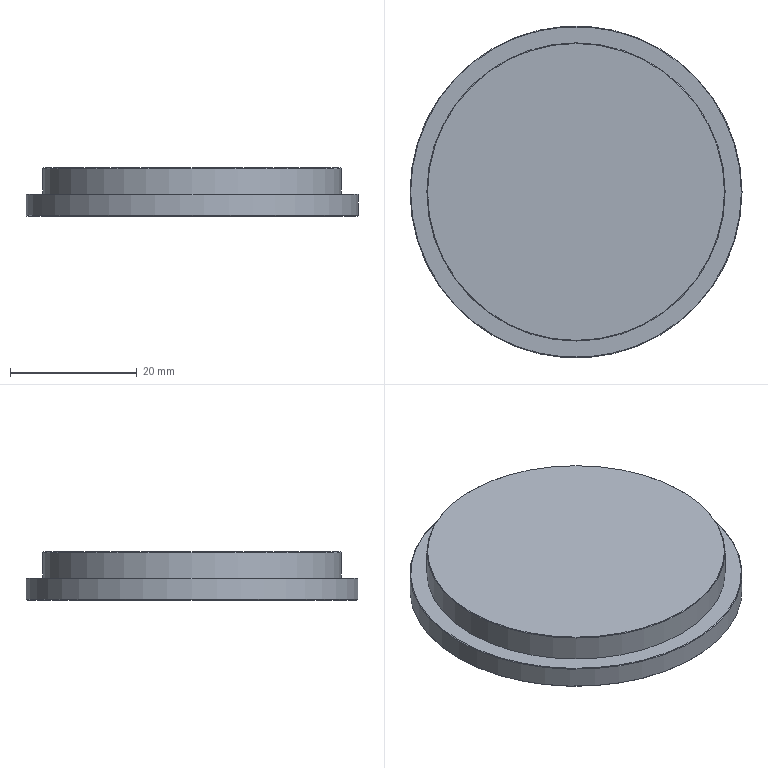Part | NX | features CHAMFER 4, DATUM_CSYS 4, EXTRUDE 3, SKETCH 3, DATUM_PLANE 2 | 1 solid | 11 faces | box 52.42 x 52.42 x 7.62 mm | volume 11135 mm3 | plane 4 | cone 4 | cylinder 3 | commonest cylinder face diameters 36.4 x1 47.08 x1 52.42 x1
STEP:
#1=CARTESIAN_POINT('',(-26.21,0.,0.1));
#2=VERTEX_POINT('',#1);
#3=CARTESIAN_POINT('',(0.,0.,0.1));
#4=DIRECTION('',(0.,0.,-1.));
#5=DIRECTION('',(-1.,0.,0.));
#6=AXIS2_PLACEMENT_3D('',#3,#4,#5);
#7=CIRCLE('',#6,26.21);
#8=EDGE_CURVE('',#2,#2,#7,.F.);
#9=ORIENTED_EDGE('',*,*,#8,.T.);
#10=EDGE_LOOP('',(#9));
#11=FACE_BOUND('',#10,.T.);
#12=CARTESIAN_POINT('',(-26.21,0.,3.38));
#13=VERTEX_POINT('',#12);
#14=CARTESIAN_POINT('',(0.,0.,3.38));
#15=DIRECTION('',(0.,0.,-1.));
#16=DIRECTION('',(-1.,0.,0.));
#17=AXIS2_PLACEMENT_3D('',#14,#15,#16);
#18=CIRCLE('',#17,26.21);
#19=EDGE_CURVE('',#13,#13,#18,.T.);
#20=ORIENTED_EDGE('',*,*,#19,.T.);
#21=EDGE_LOOP('',(#20));
#22=FACE_BOUND('',#21,.T.);
#23=CARTESIAN_POINT('',(0.,0.,7.62));
#24=DIRECTION('',(0.,0.,-1.));
#25=DIRECTION('',(-1.,0.,0.));
#26=AXIS2_PLACEMENT_3D('',#23,#24,#25);
#27=CYLINDRICAL_SURFACE('',#26,26.21);
#28=ADVANCED_FACE('',(#11,#22),#27,.T.);
#29=CARTESIAN_POINT('',(-18.3,0.,0.));
#30=VERTEX_POINT('',#29);
#31=CARTESIAN_POINT('',(0.,0.,0.));
#32=DIRECTION('',(0.,0.,-1.));
#33=DIRECTION('',(-1.,0.,0.));
#34=AXIS2_PLACEMENT_3D('',#31,#32,#33);
#35=CIRCLE('',#34,18.3);
#36=EDGE_CURVE('',#30,#30,#35,.F.);
#37=ORIENTED_EDGE('',*,*,#36,.T.);
#38=EDGE_LOOP('',(#37));
#39=FACE_BOUND('',#38,.T.);
#40=CARTESIAN_POINT('',(-26.11,0.,0.));
#41=VERTEX_POINT('',#40);
#42=CARTESIAN_POINT('',(0.,0.,0.));
#43=DIRECTION('',(0.,0.,-1.));
#44=DIRECTION('',(-1.,0.,0.));
#45=AXIS2_PLACEMENT_3D('',#42,#43,#44);
#46=CIRCLE('',#45,26.11);
#47=EDGE_CURVE('',#41,#41,#46,.T.);
#48=ORIENTED_EDGE('',*,*,#47,.T.);
#49=EDGE_LOOP('',(#48));
#50=FACE_BOUND('',#49,.T.);
#51=CARTESIAN_POINT('',(0.,0.,0.));
#52=DIRECTION('',(0.,0.,-1.));
#53=DIRECTION('',(-1.,0.,0.));
#54=AXIS2_PLACEMENT_3D('',#51,#52,#53);
#55=PLANE('',#54);
#56=ADVANCED_FACE('',(#39,#50),#55,.T.);
#57=CARTESIAN_POINT('',(-23.54,0.,7.52));
#58=VERTEX_POINT('',#57);
#59=CARTESIAN_POINT('',(0.,0.,7.52));
#60=DIRECTION('',(0.,0.,-1.));
#61=DIRECTION('',(-1.,0.,0.));
#62=AXIS2_PLACEMENT_3D('',#59,#60,#61);
#63=CIRCLE('',#62,23.54);
#64=EDGE_CURVE('',#58,#58,#63,.T.);
#65=ORIENTED_EDGE('',*,*,#64,.T.);
#66=EDGE_LOOP('',(#65));
#67=FACE_BOUND('',#66,.T.);
#68=CARTESIAN_POINT('',(23.54,0.,3.48));
#69=VERTEX_POINT('',#68);
#70=CARTESIAN_POINT('',(0.,0.,3.48));
#71=DIRECTION('',(0.,0.,-1.));
#72=DIRECTION('',(1.,0.,0.));
#73=AXIS2_PLACEMENT_3D('',#70,#71,#72);
#74=CIRCLE('',#73,23.54);
#75=EDGE_CURVE('',#69,#69,#74,.F.);
#76=ORIENTED_EDGE('',*,*,#75,.T.);
#77=EDGE_LOOP('',(#76));
#78=FACE_BOUND('',#77,.T.);
#79=CARTESIAN_POINT('',(0.,0.,3.48));
#80=DIRECTION('',(0.,0.,1.));
#81=DIRECTION('',(1.,0.,0.));
#82=AXIS2_PLACEMENT_3D('',#79,#80,#81);
#83=CYLINDRICAL_SURFACE('',#82,23.54);
#84=ADVANCED_FACE('',(#67,#78),#83,.T.);
#85=CARTESIAN_POINT('',(-26.11,0.,3.48));
#86=VERTEX_POINT('',#85);
#87=CARTESIAN_POINT('',(0.,0.,3.48));
#88=DIRECTION('',(0.,0.,-1.));
#89=DIRECTION('',(-1.,0.,0.));
#90=AXIS2_PLACEMENT_3D('',#87,#88,#89);
#91=CIRCLE('',#90,26.11);
#92=EDGE_CURVE('',#86,#86,#91,.F.);
#93=ORIENTED_EDGE('',*,*,#92,.T.);
#94=EDGE_LOOP('',(#93));
#95=FACE_BOUND('',#94,.T.);
#96=ORIENTED_EDGE('',*,*,#75,.F.);
#97=EDGE_LOOP('',(#96));
#98=FACE_BOUND('',#97,.T.);
#99=CARTESIAN_POINT('',(0.,0.,3.48));
#100=DIRECTION('',(0.,0.,-1.));
#101=DIRECTION('',(-1.,0.,0.));
#102=AXIS2_PLACEMENT_3D('',#99,#100,#101);
#103=PLANE('',#102);
#104=ADVANCED_FACE('',(#95,#98),#103,.F.);
#105=CARTESIAN_POINT('',(-23.44,0.,7.62));
#106=VERTEX_POINT('',#105);
#107=CARTESIAN_POINT('',(0.,0.,7.62));
#108=DIRECTION('',(0.,0.,-1.));
#109=DIRECTION('',(-1.,0.,0.));
#110=AXIS2_PLACEMENT_3D('',#107,#108,#109);
#111=CIRCLE('',#110,23.44);
#112=EDGE_CURVE('',#106,#106,#111,.F.);
#113=ORIENTED_EDGE('',*,*,#112,.T.);
#114=EDGE_LOOP('',(#113));
#115=FACE_BOUND('',#114,.T.);
#116=CARTESIAN_POINT('',(0.,0.,7.62));
#117=DIRECTION('',(0.,0.,-1.));
#118=DIRECTION('',(-1.,0.,0.));
#119=AXIS2_PLACEMENT_3D('',#116,#117,#118);
#120=PLANE('',#119);
#121=ADVANCED_FACE('',(#115),#120,.F.);
#122=CARTESIAN_POINT('',(-18.2,0.,0.1));
#123=VERTEX_POINT('',#122);
#124=CARTESIAN_POINT('',(0.,0.,0.1));
#125=DIRECTION('',(0.,0.,-1.));
#126=DIRECTION('',(-1.,0.,0.));
#127=AXIS2_PLACEMENT_3D('',#124,#125,#126);
#128=CIRCLE('',#127,18.2);
#129=EDGE_CURVE('',#123,#123,#128,.T.);
#130=ORIENTED_EDGE('',*,*,#129,.T.);
#131=EDGE_LOOP('',(#130));
#132=FACE_BOUND('',#131,.T.);
#133=CARTESIAN_POINT('',(18.2,0.,3.44));
#134=VERTEX_POINT('',#133);
#135=CARTESIAN_POINT('',(0.,0.,3.44));
#136=DIRECTION('',(0.,0.,1.));
#137=DIRECTION('',(1.,0.,0.));
#138=AXIS2_PLACEMENT_3D('',#135,#136,#137);
#139=CIRCLE('',#138,18.2);
#140=EDGE_CURVE('',#134,#134,#139,.F.);
#141=ORIENTED_EDGE('',*,*,#140,.F.);
#142=EDGE_LOOP('',(#141));
#143=FACE_BOUND('',#142,.T.);
#144=CARTESIAN_POINT('',(0.,0.,3.44));
#145=DIRECTION('',(0.,0.,-1.));
#146=DIRECTION('',(-1.,0.,0.));
#147=AXIS2_PLACEMENT_3D('',#144,#145,#146);
#148=CYLINDRICAL_SURFACE('',#147,18.2);
#149=ADVANCED_FACE('',(#132,#143),#148,.F.);
#150=ORIENTED_EDGE('',*,*,#140,.T.);
#151=EDGE_LOOP('',(#150));
#152=FACE_BOUND('',#151,.T.);
#153=CARTESIAN_POINT('',(0.,0.,3.44));
#154=DIRECTION('',(0.,0.,1.));
#155=DIRECTION('',(1.,0.,0.));
#156=AXIS2_PLACEMENT_3D('',#153,#154,#155);
#157=PLANE('',#156);
#158=ADVANCED_FACE('',(#152),#157,.F.);
#159=ORIENTED_EDGE('',*,*,#112,.F.);
#160=EDGE_LOOP('',(#159));
#161=FACE_BOUND('',#160,.T.);
#162=ORIENTED_EDGE('',*,*,#64,.F.);
#163=EDGE_LOOP('',(#162));
#164=FACE_BOUND('',#163,.T.);
#165=CARTESIAN_POINT('',(0.,0.,7.52));
#166=DIRECTION('',(0.,0.,-1.));
#167=DIRECTION('',(-1.,0.,0.));
#168=AXIS2_PLACEMENT_3D('',#165,#166,#167);
#169=CONICAL_SURFACE('',#168,23.54,0.7854);
#170=ADVANCED_FACE('',(#161,#164),#169,.T.);
#171=ORIENTED_EDGE('',*,*,#92,.F.);
#172=EDGE_LOOP('',(#171));
#173=FACE_BOUND('',#172,.T.);
#174=ORIENTED_EDGE('',*,*,#19,.F.);
#175=EDGE_LOOP('',(#174));
#176=FACE_BOUND('',#175,.T.);
#177=CARTESIAN_POINT('',(0.,0.,3.38));
#178=DIRECTION('',(0.,0.,-1.));
#179=DIRECTION('',(-1.,0.,0.));
#180=AXIS2_PLACEMENT_3D('',#177,#178,#179);
#181=CONICAL_SURFACE('',#180,26.21,0.7854);
#182=ADVANCED_FACE('',(#173,#176),#181,.T.);
#183=ORIENTED_EDGE('',*,*,#8,.F.);
#184=EDGE_LOOP('',(#183));
#185=FACE_BOUND('',#184,.T.);
#186=ORIENTED_EDGE('',*,*,#47,.F.);
#187=EDGE_LOOP('',(#186));
#188=FACE_BOUND('',#187,.T.);
#189=CARTESIAN_POINT('',(0.,0.,0.));
#190=DIRECTION('',(0.,0.,1.));
#191=DIRECTION('',(1.,0.,0.));
#192=AXIS2_PLACEMENT_3D('',#189,#190,#191);
#193=CONICAL_SURFACE('',#192,26.11,0.7854);
#194=ADVANCED_FACE('',(#185,#188),#193,.T.);
#195=ORIENTED_EDGE('',*,*,#129,.F.);
#196=EDGE_LOOP('',(#195));
#197=FACE_BOUND('',#196,.T.);
#198=ORIENTED_EDGE('',*,*,#36,.F.);
#199=EDGE_LOOP('',(#198));
#200=FACE_BOUND('',#199,.T.);
#201=CARTESIAN_POINT('',(0.,0.,0.));
#202=DIRECTION('',(0.,0.,-1.));
#203=DIRECTION('',(-1.,0.,0.));
#204=AXIS2_PLACEMENT_3D('',#201,#202,#203);
#205=CONICAL_SURFACE('',#204,18.3,0.7854);
#206=ADVANCED_FACE('',(#197,#200),#205,.F.);
#207=CLOSED_SHELL('',(#28,#56,#84,#104,#121,#149,#158,#170,#182,#194,#206));
#208=MANIFOLD_SOLID_BREP('',#207);
#209=(LENGTH_UNIT()NAMED_UNIT(*)SI_UNIT(.MILLI.,.METRE.));
#210=UNCERTAINTY_MEASURE_WITH_UNIT(LENGTH_MEASURE(0.00001),#209,'','');
#211=(NAMED_UNIT(*)PLANE_ANGLE_UNIT()SI_UNIT($,.RADIAN.));
#212=(NAMED_UNIT(*)SI_UNIT($,.STERADIAN.)SOLID_ANGLE_UNIT());
#213=(GEOMETRIC_REPRESENTATION_CONTEXT(3)GLOBAL_UNCERTAINTY_ASSIGNED_CONTEXT((#210))GLOBAL_UNIT_ASSIGNED_CONTEXT((#209,#211,#212))REPRESENTATION_CONTEXT('',''));
#214=ADVANCED_BREP_SHAPE_REPRESENTATION('',(#208),#213);